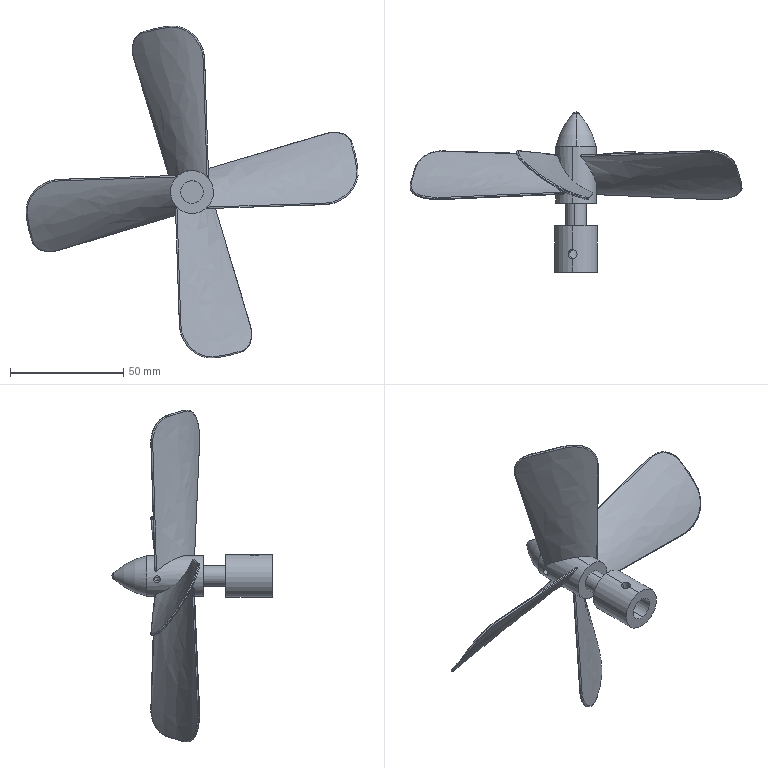Part | SolidWorks | 3 solids | 89 faces | box 146.733 x 70.903 x 146.733 mm | volume 21396 mm3 | spline 48 | cylinder 26 | plane 11 | torus 4 | commonest cylinder face diameters 3 x6 5 x4 8 x4 9.26 x4 4 x2 10 x2